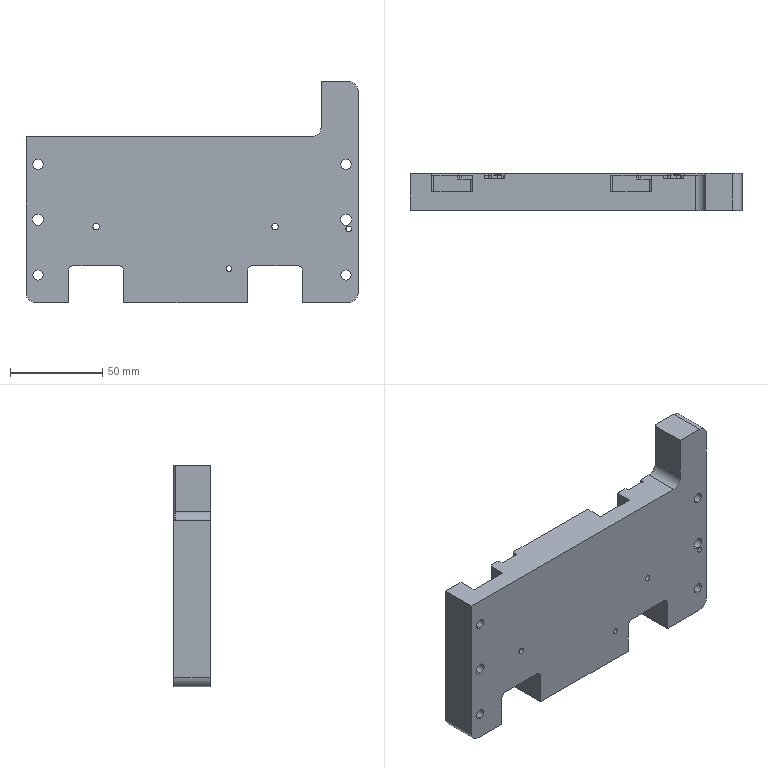Part | STEP file | 05-03 left bending base die | 1 solid | 444 faces | box 180 x 20 x 120 mm | volume 280278 mm3 | plane 189 | cylinder 176 | cone 51 | torus 20 | sphere 8 | commonest cylinder face diameters 2 x68 3 x22 4 x14 2.5 x12 3.1 x12 10 x12